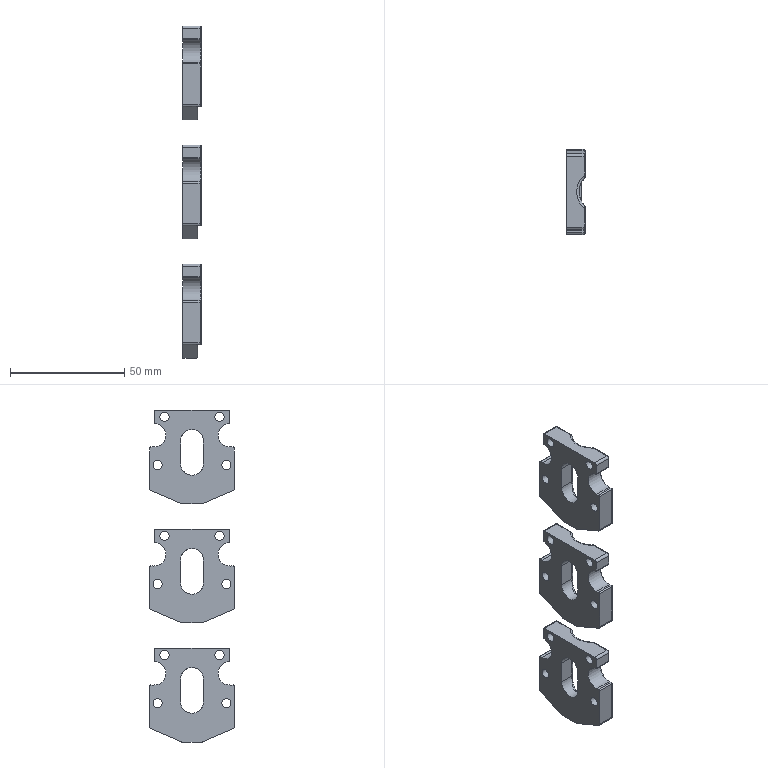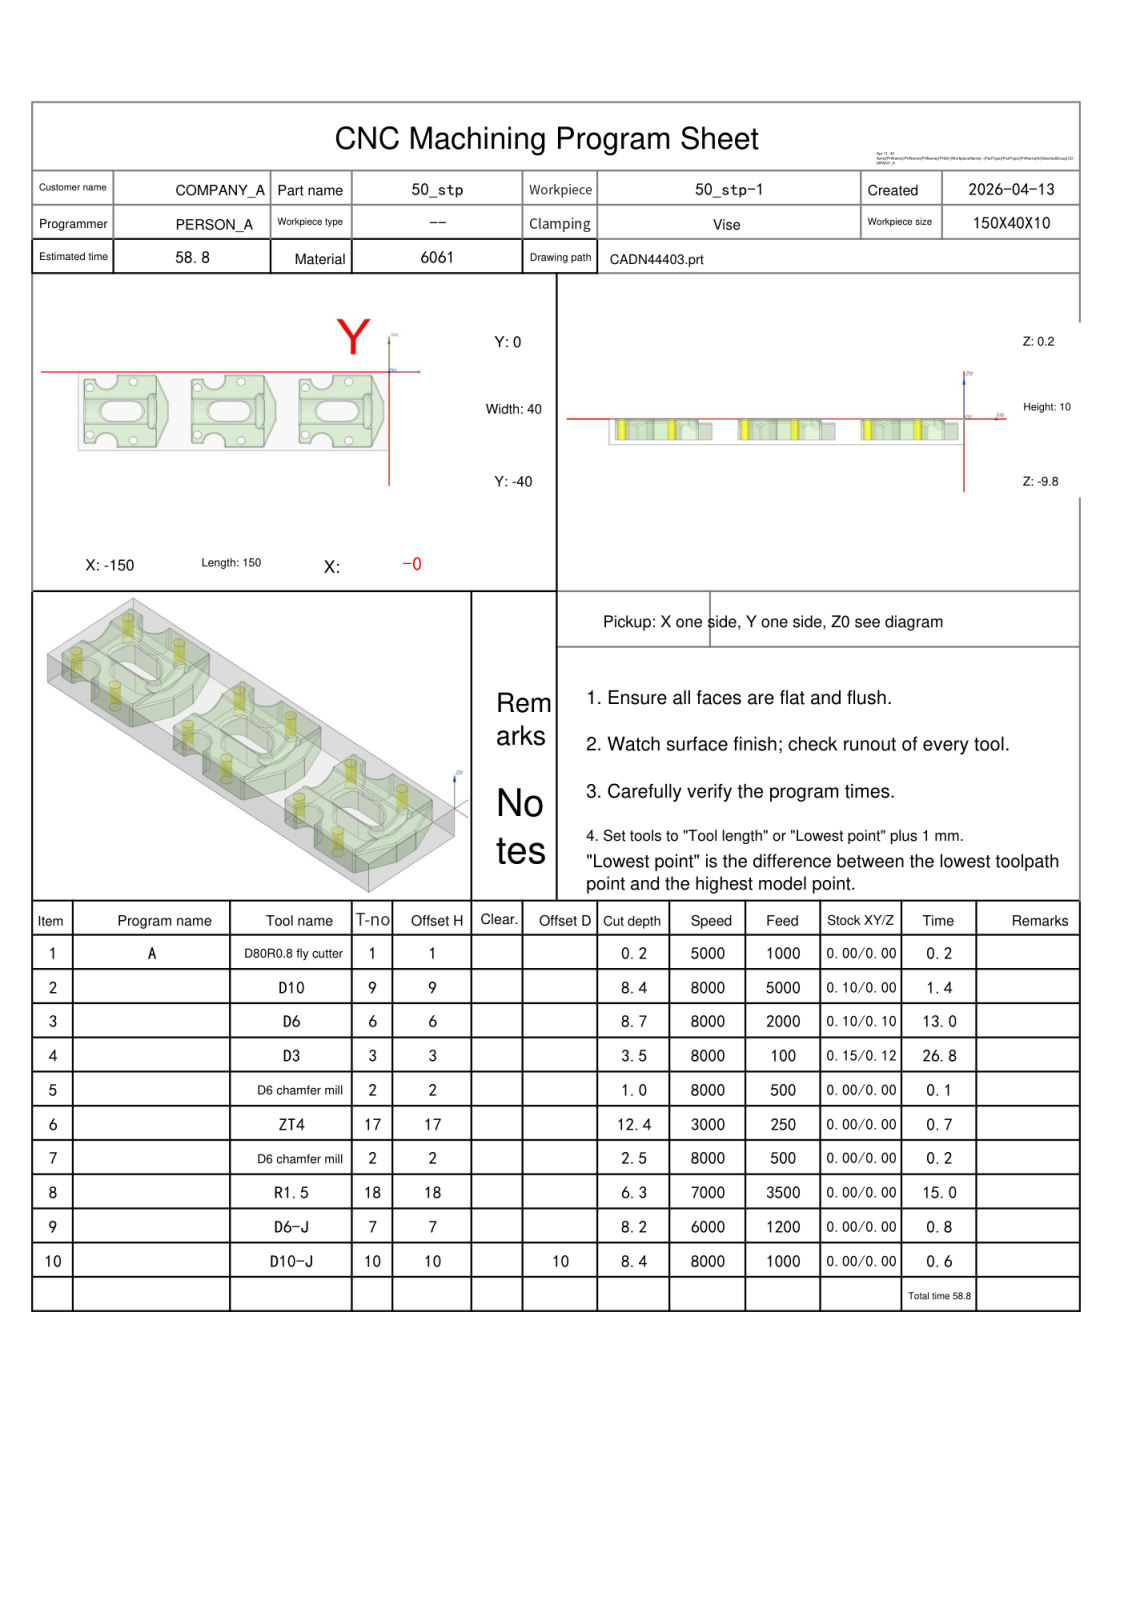NC program | NX | posted by the shop | part box 8 x 37 x 145 mm
Lines 1272 to 2331 of 223411:
N3 T06 M06
(D6  D=6. R=0. H=06 ce=0.10 di=0.10)
G00 G90 G54 X4.879 Y-15.796 M03 S8000
G43 H06 Z10.2
M08
Z.975
G01 Z-.225 F2000.
X4.5
G03 X.3 Y-19.996 I0.0 J-4.2
G01 Y-26.039
X.081 Y-26.55
X-.11 Y-26.995
G02 X-.397 Y-27.298 I-.551 J.236
G01 X-1.104 Y-27.644
G03 X-1.398 Y-27.963 I.264 J-.539
G02 X-2.795 Y-28.916 I-1.396 J.548
X-4.287 Y-27.567 I0.0 J1.5
G01 X-4.66 Y-23.887
X-4.667 Y-23.736
G02 X-3.167 Y-22.236 I1.5 J0.0
X-1.675 Y-23.585 I0.0 J-1.5
G01 X-1.365 Y-26.646
G03 X-1.289 Y-26.883 I.597 J.06
G01 X-.736 Y-27.851
G02 X-.657 Y-28.148 I-.521 J-.298
X-.705 Y-28.385 I-.6 J0.0
G01 X-5.211 Y-38.898
G02 X-5.718 Y-39.859 I-4.039 J1.518
G01 X-5.831 Y-39.78
G03 X-5.688 Y-39.553 I-3.328 J2.279
X-5.198 Y-37.615 I-3.592 J1.938
G01 X-5.2 Y-37.496
Y-29.121
X-5.197 Y-28.968
G03 X-8.5 Y-25.605 I-3.364 J0.0
G01 X-9.376
G03 X-12.749 Y-22.954 I-3.424 J-.885
G01 X-13.466
G02 X-14.063 Y-22.41 I0.0 J.6
G01 X-14.138 Y-21.619
G03 X-14.373 Y-21.197 I-.597 J-.056
G02 X-14.967 Y-20. I.905 J1.196
X-13.469 Y-18.5 I1.5 J0.0
G01 X-9.73 Y-18.497
X-9.729
G02 X-8.229 Y-19.997 I0.0 J-1.5
X-9.728 Y-21.497 I-1.5 J0.0
G01 X-12.219 Y-21.499
G03 X-12.812 Y-22.015 I.001 J-.6
G01 X-12.872 Y-22.438
G02 X-13.466 Y-22.954 I-.594 J.084
G01 X-42.586
G03 X-44.298 Y-23.405 I0.0 J-3.472
X-46.53 Y-27.082 I2.172 J-3.836
G01 X-46.68
Y-27.077
Y-24.633
Y-13.139
Y-12.918
X-46.528
X-46.525 Y-12.967
X-46.37 Y-13.961
X-46.025 Y-14.751
G03 X-42.975 Y-17.019 I3.509 J1.534
G02 X-42.447 Y-17.614 I-.072 J-.596
X-42.518 Y-17.898 I-.6 J0.0
G01 X-42.978 Y-18.756
G03 X-43.042 Y-19.011 I.476 J-.255
X-42.85 Y-19.424 I.54 J0.0
G02 X-42.584 Y-19.997 I-.484 J-.573
X-43.247 Y-20.742 I-.75 J0.0
G03 X-43.553 Y-20.786 I.661 J-5.684
G01 X-43.68 Y-20.797
G02 X-44.43 Y-20.047 I0.0 J.75
G01 Y-19.946
G02 X-44.312 Y-19.543 I.75 J0.0
G01 X-44.247 Y-19.403
X-43.618 Y-17.432
G02 X-43.047 Y-17.014 I.572 J-.182
G01 X-42.975 Y-17.019
G03 X-42.516 Y-17.046 I.459 J3.802
G01 X-12.749
G03 X-9.362 Y-14.395 I-.07 J3.579
G01 X-8.5
G03 X-5.199 Y-11.013 I-.081 J3.381
G01 X-5.2 Y-10.932
Y-2.504
X-5.198 Y-2.367
G03 X-5.689 Y-.445 I-4.005 J0.0
X-5.831 Y-.221 I-3.47 J-2.055
G01 X-5.731 Y-.149
G02 X-5.212 Y-1.101 I-3.568 J-2.562
G01 X-.712 Y-11.599
G02 X-.664 Y-11.835 I-.551 J-.236
X-.743 Y-12.133 I-.6 J0.0
G01 X-1.296 Y-13.102
G03 X-1.372 Y-13.341 I.521 J-.297
G01 X-1.672 Y-16.401
G02 X-3.165 Y-17.755 I-1.493 J.147
X-4.665 Y-16.255 I0.0 J1.5
G01 X-4.658 Y-16.108
X-4.296 Y-12.427
G02 X-2.804 Y-11.073 I1.493 J-.147
X-1.409 Y-12.021 I0.0 J-1.5
G03 X-1.115 Y-12.34 I.558 J.221
G01 X-.404 Y-12.687
G02 X-.116 Y-12.99 I-.264 J-.539
G01 X.228 Y-13.793
X.3 Y-13.961
Y-20.966
G02 X-.226 Y-21.561 I-.6 J0.0
G01 X-3.593 Y-21.981
G03 X-4.009 Y-22.231 I.074 J-.595
G02 X-4.5 Y-22.486 I-.491 J.345
X-4.797 Y-22.407 I0.0 J.6
G03 X-6.613 Y-21.659 I-3.763 J-6.561
G02 X-6.912 Y-21.471 I.156 J.579
G03 X-7.947 Y-20.465 I-5.888 J-5.019
G02 X-8.169 Y-19.998 I.378 J.466
X-7.946 Y-19.532 I.6 J0.0
G03 X-6.906 Y-18.522 I-4.873 J6.065
G02 X-6.608 Y-18.335 I.455 J-.391
G03 X-4.798 Y-17.584 I-1.973 J7.321
G02 X-4.5 Y-17.505 I.298 J-.521
X-3.9 Y-18.104 I0.0 J-.6
G01 Y-21.887
X-3.915 Y-22.021
G02 X-4.207 Y-22.409 I-.585 J.135
G03 X-5.281 Y-24.242 I1.026 J-1.833
X-5.014 Y-25.267 I2.1 J0.0
G01 X4.579 Y-26.509
Z.975
G00 Z3.
G01 X4.879 Y-15.797 F6000.
G00 Z.75
G01 Z-.45 F2000.
X4.5
G03 X.3 Y-19.997 I0.0 J-4.2
G01 Y-26.039
X.081 Y-26.55
X-.382 Y-27.631
G02 X-.701 Y-27.932 I-.506 J.217
G01 X-1.361 Y-28.171
G03 X-1.597 Y-28.327 I.205 J-.564
G02 X-2.698 Y-28.809 I-1.101 J1.018
X-4.184 Y-27.516 I0.0 J1.5
G01 X-4.705 Y-23.77
G02 X-4.72 Y-23.564 I1.486 J.207
X-3.22 Y-22.064 I1.5 J0.0
X-1.734 Y-23.357 I0.0 J-1.5
G01 X-1.213 Y-27.102
G02 X-1.198 Y-27.309 I-1.486 J-.207
G01 X-1.202 Y-27.413
X-1.203 Y-27.451
G03 X-1.157 Y-27.672 I.55 J0.0
G01 X-.879 Y-28.307
G02 X-.828 Y-28.548 I-.549 J-.241
X-.876 Y-28.784 I-.6 J0.0
G01 X-5.211 Y-38.898
G02 X-5.718 Y-39.859 I-4.039 J1.518
G01 X-5.778 Y-39.817
X-5.776 Y-39.811
G03 X-5.2 Y-37.947 I-2.731 J1.864
G01 Y-37.946
Y-37.734
X-5.198 Y-37.615
X-5.2 Y-37.496
Y-29.121
X-5.196 Y-28.964
X-5.2 Y-28.808
Y-28.772
G03 X-8.5 Y-25.436 I-3.336 J0.0
G01 X-9.313
G03 X-12.749 Y-22.707 I-3.483 J-.858
G01 X-42.586
G03 X-45.021 Y-23.656 I0.0 J-3.6
X-46.595 Y-27.082 I3.297 J-3.59
G01 X-46.68 Y-27.079
Y-24.401
Y-13.139
Y-12.918
X-46.595
G03 X-45.73 Y-15.54 I4.991 J.192
X-42.5 Y-17.293 I3.259 J2.154
G01 X-12.749
G03 X-9.315 Y-14.564 I-.039 J3.574
G01 X-8.5
G03 X-6.884 Y-14.121 I-.048 J3.348
X-5.198 Y-11.213 I-1.664 J2.908
G01 X-5.2 Y-11.095
Y-10.932
Y-2.504
X-5.198 Y-2.367
X-5.2 Y-2.23
Y-2.054
Y-2.053
G03 X-5.779 Y-.184 I-3.307 J0.0
G01 X-5.731 Y-.149
G02 X-5.212 Y-1.101 I-3.568 J-2.562
G01 X-.871 Y-11.228
G02 X-.827 Y-11.445 I-.507 J-.217
X-.873 Y-11.667 I-.551 J0.0
G01 X-1.156 Y-12.312
G03 X-1.207 Y-12.553 I.55 J-.241
G01 X-1.206 Y-12.591
X-1.203 Y-12.685
G02 X-1.217 Y-12.89 I-1.5 J0.0
G01 X-1.733 Y-16.636
G02 X-3.219 Y-17.931 I-1.486 J.205
X-4.719 Y-16.431 I0.0 J1.5
X-4.705 Y-16.226 I1.5 J0.0
G01 X-4.189 Y-12.481
G02 X-2.703 Y-11.185 I1.486 J-.205
X-1.596 Y-11.673 I0.0 J-1.5
G03 X-1.377 Y-11.819 I.407 J.372
G01 X-.723 Y-12.056
G02 X-.376 Y-12.383 I-.205 J-.564
G01 X.228 Y-13.793
X.3 Y-13.961
Y-22.997
G02 X-.3 Y-23.597 I-.6 J0.0
X-.568 Y-23.534 I0.0 J.6
G01 X-3.463 Y-22.091
G03 X-3.73 Y-22.028 I-.267 J-.537
X-4.115 Y-22.168 I0.0 J-.6
G02 X-4.5 Y-22.308 I-.385 J.46
X-4.796 Y-22.229 I0.0 J.6
G03 X-6.506 Y-21.515 I-3.74 J-6.543
G02 X-6.804 Y-21.322 I.163 J.577
G03 X-7.65 Y-20.451 I-5.993 J-4.973
G02 X-7.852 Y-20.001 I.398 J.449
X-7.65 Y-19.552 I.6 J0.0
G03 X-6.798 Y-18.674 I-5.139 J5.834
G02 X-6.501 Y-18.481 I.461 J-.384
G03 X-4.797 Y-17.766 I-2.047 J7.266
G02 X-4.5 Y-17.687 I.297 J-.522
X-3.9 Y-18.285 I0.0 J-.6
G01 Y-21.709
X-3.921 Y-21.863
G02 X-4.226 Y-22.241 I-.579 J.156
G03 X-5.365 Y-24.109 I.96 J-1.868
X-5.133 Y-25.069 I2.1 J0.0
G01 X4.579 Y-26.509
Z.75
G00 Z2.775
G01 X4.879 Y-15.794 F6000.
G00 Z.525
G01 Z-.675 F2000.
X4.5
G03 X.3 Y-19.994 I0.0 J-4.2
G01 Y-26.039
X.081 Y-26.55
X-.345 Y-27.543
G02 X-.646 Y-27.829 I-.481 J.206
G01 X-1.265 Y-28.054
G03 X-1.504 Y-28.215 I.205 J-.564
G02 X-2.616 Y-28.708 I-1.112 J1.007
X-4.094 Y-27.458 I0.0 J1.5
G01 X-4.741 Y-23.644
G02 X-4.762 Y-23.393 I1.479 J.251
X-3.262 Y-21.893 I1.5 J0.0
X-1.783 Y-23.142 I0.0 J-1.5
G01 X-1.137 Y-26.957
G02 X-1.116 Y-27.208 I-1.479 J-.251
G01 X-1.121 Y-27.332
X-1.123 Y-27.375
G03 X-1.079 Y-27.585 I.523 J0.0
G01 X-.821 Y-28.175
G02 X-.771 Y-28.415 I-.55 J-.24
X-.819 Y-28.651 I-.6 J0.0
G01 X-5.211 Y-38.898
G02 X-5.718 Y-39.859 I-4.039 J1.518
G01 X-5.777 Y-39.818
X-5.684 Y-39.673
G03 X-5.2 Y-37.953 I-2.816 J1.72
G01 Y-37.946
Y-37.734
X-5.198 Y-37.615
X-5.2 Y-37.496
Y-29.121
X-5.196 Y-28.964
X-5.2 Y-28.808
Y-28.637
Y-28.597
G03 X-8.5 Y-25.258 I-3.34 J0.0
G01 X-9.292
G03 X-12.749 Y-22.44 I-3.556 J-.833
G01 X-42.5
X-42.519
G03 X-44.988 Y-23.362 I0.0 J-3.769
X-46.6 Y-27.068 I3.456 J-3.706
G01 Y-27.082
X-46.601
X-46.68
Y-24.169
Y-13.139
Y-12.918
X-46.6
Y-12.942
G03 X-45.562 Y-16.026 I5.254 J.052
X-42.51 Y-17.56 I3.052 J2.27
G01 X-12.749
G03 X-9.29 Y-14.742 I-.1 J3.655
G01 X-8.5
G03 X-6.89 Y-14.295 I-.071 J3.37
X-5.195 Y-11.367 I-1.68 J2.927
G01 X-5.2 Y-11.192
Y-11.095
Y-10.932
Y-2.504
X-5.198 Y-2.367
X-5.2 Y-2.23
Y-2.047
G03 X-5.641 Y-.403 I-3.3 J-.004
G01 X-5.777 Y-.183
X-5.728 Y-.152
G02 X-5.212 Y-1.101 I-3.571 J-2.559
G01 X-.814 Y-11.363
G02 X-.771 Y-11.57 I-.483 J-.207
X-.815 Y-11.78 I-.526 J0.0
G01 X-1.08 Y-12.387
G03 X-1.13 Y-12.627 I.55 J-.24
G01 X-1.129 Y-12.67
X-1.125 Y-12.78
G02 X-1.145 Y-13.026 I-1.5 J0.0
G01 X-1.781 Y-16.841
G02 X-3.26 Y-18.094 I-1.48 J.246
X-4.76 Y-16.594 I0.0 J1.5
X-4.74 Y-16.348 I1.5 J0.0
G01 X-4.104 Y-12.533
G02 X-2.625 Y-11.28 I1.48 J-.246
X-1.505 Y-11.782 I0.0 J-1.5
G03 X-1.292 Y-11.926 I.392 J.35
G01 X-.683 Y-12.147
G02 X-.337 Y-12.475 I-.205 J-.564
G01 X.228 Y-13.793
X.3 Y-13.961
Y-22.994
G02 X-.3 Y-23.594 I-.6 J0.0
X-.587 Y-23.521 I0.0 J.6
G01 X-3.476 Y-21.95
G03 X-3.763 Y-21.877 I-.286 J-.527
X-4.131 Y-22.004 I0.0 J-.6
G02 X-4.5 Y-22.131 I-.369 J.473
X-4.796 Y-22.052 I0.0 J.6
G03 X-6.442 Y-21.355 I-3.743 J-6.545
G02 X-6.739 Y-21.158 I.169 J.576
G03 X-7.405 Y-20.431 I-6.109 J-4.933
G02 X-7.588 Y-20. I.417 J.431
X-7.405 Y-19.569 I.6 J0.0
G03 X-6.732 Y-18.833 I-5.445 J5.664
G02 X-6.437 Y-18.636 I.466 J-.378
G03 X-4.797 Y-17.936 I-2.134 J7.264
G02 X-4.5 Y-17.857 I.297 J-.521
X-3.9 Y-18.455 I0.0 J-.6
G01 Y-21.532
X-3.926 Y-21.705
G02 X-4.244 Y-22.073 I-.574 J.175
G03 X-5.446 Y-23.972 I.897 J-1.899
X-5.245 Y-24.869 I2.1 J0.0
G01 X4.579 Y-26.509
Z.525
G00 Z2.55
G01 X4.879 Y-15.8 F6000.
G00 Z.3
G01 Z-.9 F2000.
X4.5
G03 X.3 Y-20. I0.0 J-4.2
G01 Y-26.039
X.081 Y-26.55
X-.3 Y-27.439
G02 X-.587 Y-27.71 I-.458 J.196
G01 X-1.166 Y-27.922
G03 X-1.408 Y-28.087 I.206 J-.563
G02 X-2.529 Y-28.59 I-1.121 J.996
X-4. Y-27.382 I0.0 J1.5
G01 X-4.774 Y-23.478
G02 X-4.803 Y-23.186 I1.471 J.292
X-3.303 Y-21.686 I1.5 J0.0
X-1.832 Y-22.894 I0.0 J-1.5
G01 X-1.058 Y-26.799
G02 X-1.029 Y-27.09 I-1.471 J-.292
G01 X-1.036 Y-27.234
X-1.038 Y-27.282
G03 X-.997 Y-27.481 I.498 J0.0
G01 X-.758 Y-28.029
G02 X-.708 Y-28.269 I-.55 J-.239
X-.757 Y-28.505 I-.6 J0.0
G01 X-5.211 Y-38.898
G02 X-5.715 Y-39.854 I-4.039 J1.518
G01 X-5.773 Y-39.813
X-5.684 Y-39.673
G03 X-5.2 Y-37.953 I-2.816 J1.72
G01 Y-37.946
Y-28.459
X-5.199 Y-28.396
G03 X-8.5 Y-25.033 I-3.363 J0.0
G01 X-9.28
G03 X-12.749 Y-22.15 I-3.574 J-.771
G01 X-18.484
X-20. Y-22.182
X-30.
X-31.516 Y-22.15
X-42.5
G03 X-45.6 Y-23.774 I.001 J-3.773
X-45.723 Y-23.951 I4.28 J-3.092
X-46.6 Y-26.854 I4.403 J-2.914
G01 X-46.68
Y-23.911
Y-13.145
X-46.6
Y-13.184
G03 X-45.6 Y-16.226 I5.283 J.05
X-42.5 Y-17.85 I3.101 J2.149
G01 X-31.516
X-30. Y-17.818
X-20.
X-18.484 Y-17.85
X-12.749
G03 X-9.28 Y-14.967 I-.077 J3.622
G01 X-8.5
G03 X-5.199 Y-11.604 I-.063 J3.363
G01 X-5.2 Y-11.541
Y-2.047
G03 X-5.615 Y-.445 I-3.3 J0.0
G01 X-5.774 Y-.188
X-5.725 Y-.157
G02 X-5.212 Y-1.101 I-3.574 J-2.554
G01 X-.74 Y-11.535
G02 X-.699 Y-11.731 I-.458 J-.196
X-.741 Y-11.93 I-.498 J0.0
G01 X-.987 Y-12.496
G03 X-1.036 Y-12.735 I.55 J-.239
G01 X-1.034 Y-12.785
X-1.029 Y-12.91
G02 X-1.058 Y-13.201 I-1.5 J0.0
G01 X-1.832 Y-17.106
G02 X-3.303 Y-18.314 I-1.471 J.292
X-4.803 Y-16.814 I0.0 J1.5
X-4.774 Y-16.522 I1.5 J0.0
G01 X-4. Y-12.618
G02 X-2.529 Y-11.41 I1.471 J-.292
X-1.395 Y-11.927 I0.0 J-1.5
G03 X-1.19 Y-12.069 I.377 J.326
G01 X-.628 Y-12.275
G02 X-.283 Y-12.602 I-.206 J-.563
G01 X.228 Y-13.793
X.3 Y-13.961
Y-23.
G02 X-.3 Y-23.6 I-.6 J0.0
X-.609 Y-23.514 I0.0 J.6
G01 X-3.494 Y-21.778
G03 X-3.804 Y-21.693 I-.309 J-.514
X-4.152 Y-21.804 I0.0 J-.6
G02 X-4.5 Y-21.915 I-.348 J.489
X-4.797 Y-21.837 I0.0 J.6
G03 X-6.38 Y-21.154 I-3.766 J-6.559
G02 X-6.675 Y-20.953 I.175 J.574
G03 X-7.137 Y-20.416 I-6.179 J-4.851
G02 X-7.299 Y-20.006 I.438 J.41
X-7.137 Y-19.596 I.6 J0.0
G03 X-6.662 Y-19.044 I-5.69 J5.368
G02 X-6.367 Y-18.842 I.471 J-.371
G03 X-4.797 Y-18.163 I-2.196 J7.238
G02 X-4.5 Y-18.085 I.297 J-.521
X-3.9 Y-18.682 I0.0 J-.6
G01 Y-21.318
G02 X-3.934 Y-21.514 I-.6 J.002
X-4.266 Y-21.868 I-.566 J.199
G03 X-5.549 Y-23.802 I.818 J-1.934
X-5.383 Y-24.62 I2.1 J0.0
G01 X4.579 Y-26.509
Z.3
G00 Z2.325
G01 X4.879 Y-15.79 F6000.
G00 Z.075
G01 Z-1.125 F2000.
X4.5
G03 X.3 Y-19.99 I0.0 J-4.2
G01 Y-26.039
X.081 Y-26.55
X-.233 Y-27.284
G02 X-.505 Y-27.542 I-.435 J.187
G01 X-1.046 Y-27.74
G03 X-1.291 Y-27.909 I.207 J-.563
G02 X-2.421 Y-28.423 I-1.131 J.986
X-3.884 Y-27.256 I0.0 J1.5
G01 X-4.808 Y-23.199
G02 X-4.845 Y-22.866 I1.463 J.333
X-3.345 Y-21.366 I1.5 J0.0
X-1.883 Y-22.533 I0.0 J-1.5
G01 X-.959 Y-26.59
G02 X-.921 Y-26.923 I-1.463 J-.333
G01 X-.93 Y-27.086
X-.933 Y-27.138
X-.894 Y-27.326
X-.674 Y-27.834
G02 X-.624 Y-28.073 I-.551 J-.239
X-.673 Y-28.309 I-.6 J0.0
G01 X-5.211 Y-38.898
G02 X-5.711 Y-39.849 I-4.039 J1.518
G01 X-5.77 Y-39.808
X-5.684 Y-39.673
G03 X-5.2 Y-37.953 I-2.816 J1.72
G01 Y-37.946
Y-28.459
X-5.199 Y-28.384
X-5.203 Y-28.231
X-5.221 Y-27.891
G03 X-8.5 Y-24.702 I-3.338 J-.153
G01 X-9.296
G03 X-12.749 Y-21.831 I-3.549 J-.757
G01 X-17.484
G02 X-20. Y-22.025 I-7.71 J83.514
G01 X-30.
X-30.481 Y-22.015
X-32.518 Y-21.831
X-42.629
G03 X-45.064 Y-22.849 I0.0 J-3.422
X-46.6 Y-26.592 I3.791 J-3.743
G01 Y-26.609
X-46.68
Y-23.626
Y-16.38
Y-13.312
X-46.6
Y-13.399
G03 X-45.529 Y-16.635 I5.54 J.04
X-42.502 Y-18.169 I3.026 J2.218
G01 X-32.516
X-30.481 Y-17.985
X-30. Y-17.975
X-20.
G02 X-17.482 Y-18.169 I-5.202 J-83.882
G01 X-12.749
G03 X-9.296 Y-15.298 I-.095 J3.628
G01 X-8.5
G03 X-5.198 Y-11.882 I-.116 J3.416
G01 X-5.2 Y-11.769
Y-2.047
G03 X-5.615 Y-.445 I-3.3 J0.0
G01 X-5.771 Y-.193
X-5.721 Y-.162
G02 X-5.212 Y-1.101 I-3.578 J-2.549
G01 X-.654 Y-11.734
X-.616 Y-11.92
X-.655 Y-12.108
X-.884 Y-12.636
G03 X-.933 Y-12.874 I.551 J-.238
G01 X-.931 Y-12.93
X-.924 Y-13.069
G02 X-.962 Y-13.403 I-1.5 J0.0
G01 X-1.885 Y-17.448
G02 X-3.347 Y-18.614 I-1.462 J.334
X-4.847 Y-17.114 I0.0 J1.5
X-4.809 Y-16.78 I1.5 J0.0
G01 X-3.886 Y-12.735
G02 X-2.424 Y-11.569 I1.462 J-.334
X-1.277 Y-12.102 I0.0 J-1.5
G03 X-1.079 Y-12.241 I.362 J.305
G01 X-.56 Y-12.432
G02 X-.215 Y-12.758 I-.207 J-.563
G01 X.228 Y-13.793
X.3 Y-13.961
Y-18.992
G02 X-.157 Y-19.575 I-.6 J0.0
G01 X-3.443 Y-20.38
G03 X-3.9 Y-20.963 I.143 J-.583
G01 Y-20.988
G02 X-4.5 Y-21.585 I-.6 J.002
X-4.797 Y-21.507 I0.0 J.6
G03 X-6.397 Y-20.818 I-3.761 J-6.537
G02 X-6.693 Y-20.617 I.174 J.574
G03 X-6.881 Y-20.387 I-6.152 J-4.842
G02 X-7.022 Y-20. I.459 J.387
X-6.881 Y-19.613 I.6 J0.0
G03 X-6.681 Y-19.368 I-5.964 J5.072
G02 X-6.388 Y-19.167 I.471 J-.372
G03 X-4.799 Y-18.474 I-2.228 J7.285
G02 X-4.5 Y-18.395 I.299 J-.52
X-3.9 Y-18.992 I0.0 J-.6
G01 Y-19.492
G03 X.3 Y-23.692 I4.2 J0.0
G01 X4.879
Z.075
G00 Z2.1
G01 Y-15.792 F6000.
G00 Z-.15
G01 Z-1.35 F2000.
X4.5
G03 X.3 Y-19.992 I0.0 J-4.2
G01 Y-26.039
X.081 Y-26.55
X0.0 Y-26.739
G02 X-.337 Y-27.057 I-.535 J.23
G01 X-1.049 Y-27.313
G03 X-1.281 Y-27.465 I.203 J-.564
G02 X-2.37 Y-27.933 I-1.089 J1.032
X-3.83 Y-26.777 I0.0 J1.5
G01 X-4.829 Y-22.539
G02 X-4.869 Y-22.194 I1.46 J.344
X-3.369 Y-20.694 I1.5 J0.0
X-1.909 Y-21.85 I0.0 J-1.5
G01 X-.91 Y-26.089
G02 X-.87 Y-26.433 I-1.46 J-.344
G01 X-.872 Y-26.513
X-.873 Y-26.543
G03 X-.823 Y-26.778 I.582 J0.0
G01 X-.519 Y-27.467
G02 X-.468 Y-27.709 I-.549 J-.242
X-.517 Y-27.945 I-.6 J0.0
G01 X-5.211 Y-38.898
G02 X-5.707 Y-39.843 I-4.039 J1.518
G01 X-5.767 Y-39.802
X-5.684 Y-39.673
G03 X-5.246 Y-38.5 I-2.816 J1.72
X-5.2 Y-37.953 I-3.254 J.547
G01 Y-37.946
Y-28.459
Y-28.333
Y-27.93
X-5.261 Y-27.204
G03 X-8.646 Y-23.979 I-3.384 J-.163
X-9.386 Y-24.061 I0.0 J-3.388
X-12.749 Y-21.496 I-3.457 J-1.045
G01 X-16.79
X-18.362 Y-21.715
X-19.44 Y-21.913
G02 X-19.737 Y-21.94 I-.298 J1.62
G01 X-30.012
G02 X-31.266 Y-21.786 I0.0 J5.172
G01 X-31.548 Y-21.715
X-33.211 Y-21.496
X-42.506
G03 X-45.302 Y-22.797 I0.0 J-3.657
X-46.6 Y-26.351 I4.219 J-3.554
G01 Y-26.357
X-46.68
Y-23.337
Y-13.643
X-46.601
X-46.6 Y-13.649
G03 X-45.302 Y-17.203 I5.517 J0.0
X-42.506 Y-18.504 I2.797 J2.356
G01 X-33.21
X-31.549 Y-18.285
X-31.266 Y-18.214
G02 X-30.01 Y-18.06 I1.256 J-5.029
G01 X-20.
G02 X-18.737 Y-18.216 I-.125 J-6.194
G01 X-18.39 Y-18.285
X-16.789 Y-18.504
X-12.749
G03 X-9.367 Y-15.894 I-.101 J3.628
G01 X-9.295 Y-15.892
X-8.866 Y-16.
X-8.5
G03 X-5.261 Y-12.796 I-.142 J3.383
G01 X-5.2 Y-12.07
Y-11.995
X-5.198 Y-11.882
X-5.2 Y-11.769
Y-2.047
G03 X-5.615 Y-.445 I-3.3 J0.0
G01 X-5.768 Y-.198
X-5.717 Y-.167
G02 X-5.212 Y-1.101 I-3.581 J-2.544
G01 X-.517 Y-12.056
G02 X-.47 Y-12.283 I-.531 J-.228
X-.519 Y-12.517 I-.578 J0.0
G01 X-.821 Y-13.202
G03 X-.872 Y-13.444 I.549 J-.242
G01 X-.871 Y-13.476
X-.869 Y-13.555
G02 X-.909 Y-13.899 I-1.5 J0.0
G01 X-1.909 Y-18.134
G02 X-3.369 Y-19.289 I-1.46 J.345
X-4.869 Y-17.789 I0.0 J1.5
X-4.829 Y-17.445 I1.5 J0.0
G01 X-3.829 Y-13.21
G02 X-2.369 Y-12.055 I1.46 J-.345
X-1.277 Y-12.527 I0.0 J-1.5
G03 X-1.051 Y-12.675 I.421 J.396
G01 X-.35 Y-12.927
G02 X-.002 Y-13.255 I-.204 J-.564
G01 X.228 Y-13.793
X.3 Y-13.961
Y-19.675
G02 X-.294 Y-20.275 I-.6 J0.0
G01 X-3.466 Y-20.305
G03 X-3.98 Y-20.605 I.006 J-.6
G02 X-4.5 Y-20.906 I-.52 J.299
X-4.802 Y-20.825 I0.0 J.6
G03 X-5.352 Y-20.531 I-3.844 J-6.542
G02 X-5.689 Y-19.992 I.263 J.539
X-5.352 Y-19.452 I.6 J0.0
G03 X-4.802 Y-19.159 I-3.291 J6.835
G02 X-4.5 Y-19.078 I.302 J-.519
X-3.9 Y-19.675 I0.0 J-.6
G01 Y-20.175
G03 X.3 Y-24.375 I4.2 J0.0
G01 X4.879
Z-.15
G00 Z1.875
G01 Y-19.992 F6000.
G00 Z-.397
G01 Z-1.597 F2000.
X.485
Y-15.603
G03 X.203 Y-14.23 I-3.485 J0.0
G01 X-5.241 Y-1.526
G03 X-5.656 Y-.379 I-3.257 J-.528
G01 X-5.764 Y-.204
X-5.713 Y-.173
G02 X-5.212 Y-1.101 I-3.585 J-2.538
G01 X.228 Y-13.793
X.3 Y-13.961
X.385 Y-14.161
X.6 Y-14.845
X.679 Y-15.54
Y-24.469
X.597 Y-25.17
X.375 Y-25.864
X.3 Y-26.039
X.081 Y-26.55
X-5.211 Y-38.898
G02 X-5.704 Y-39.838 I-4.039 J1.518
G01 X-5.763 Y-39.797
X-5.684 Y-39.673
G03 X-5.241 Y-38.474 I-2.816 J1.72
G01 X.203 Y-25.77
G03 X.485 Y-24.397 I-3.203 J1.373
G01 Y-19.992
Y-19.492
Z-.397
G00 Z1.65
G01 X4.879 Y-19.992 F6000.
G00 Z-.643
G01 Z-1.843 F2000.
X.59
Y-15.603
G03 X.3 Y-14.188 I-3.59 J0.0
G01 X-5.4 Y-.889
G03 X-5.499 Y-.674 I-3.76 J-1.611
X-5.615 Y-.445 I-3.001 J-1.373
G01 X-5.76 Y-.21
X-5.712 Y-.175
G02 X-5.212 Y-1.101 I-3.587 J-2.536
G01 X.228 Y-13.793
X.3 Y-13.961
X.385 Y-14.161
X.6 Y-14.845
X.679 Y-15.54
Y-24.469
X.597 Y-25.17
X.375 Y-25.864
X.3 Y-26.039
X.081 Y-26.55
X-5.211 Y-38.898
G02 X-5.7 Y-39.832 I-4.039 J1.518
G01 X-5.759 Y-39.791
X-5.684 Y-39.673
G03 X-5.499 Y-39.326 I-2.816 J1.72
X-5.4 Y-39.111 I-3.66 J1.826
G01 X.3 Y-25.812
G03 X.59 Y-24.397 I-3.3 J1.414
G01 Y-19.992
Y-19.492
Z-.643
G00 Z1.65
G01 X-44.4 Y-21.197 F6000.
G00 Z.15
G02 X-44.4 Y-21.197 Z-.133 I-2.28 J1.207 F2000.
X-44.4 Y-21.197 Z-.416 I-2.28 J1.207
X-44.4 Y-21.197 Z-.699 I-2.28 J1.207
X-44.4 Y-21.197 Z-.982 I-2.28 J1.207
X-44.4 Y-21.197 Z-1.265 I-2.28 J1.207
X-44.4 Y-21.197 Z-1.548 I-2.28 J1.207
X-46.68 Y-22.57 Z-1.597 I-2.28 J1.207
G01 Y-19.99
Y-13.896
X-46.601
G03 X-45.81 Y-16.912 I6.228 J.02
X-42.5 Y-18.956 I3.373 J1.76
G01 X-33.901
G03 X-31.383 Y-18.391 I-.52 J8.215
G02 X-30. Y-18.099 I1.565 J-3.991
G01 X-20.
G02 X-18.737 Y-18.355 I-.119 J-3.834
G03 X-16.099 Y-18.956 I3.328 J8.514
G01 X-12.749
X-11.395 Y-18.672
Y-21.328
X-12.749 Y-21.044
X-16.099
G03 X-18.737 Y-21.645 I.723 J-9.262
G02 X-19.999 Y-21.901 I-1.262 J2.984
G01 X-20.
X-30.
G02 X-31.382 Y-21.609 I.155 J4.153
G03 X-33.901 Y-21.044 I-3.039 J-7.65
G01 X-42.632
G03 X-45.086 Y-22.127 I0.0 J-3.322
X-46.603 Y-26.041 I4.291 J-3.915
G01 Y-26.084
X-46.68
Y-19.99
Y-19.49
G03 X-50.88 Y-15.29 I-4.2 J0.0
G01 Z-.397
G00 Z1.65
G01 X-44.712 Y-21.017 F6000.
G00 Z-.097
G02 X-44.712 Y-21.017 Z-.34 I-1.968 J1.027 F2000.
X-44.712 Y-21.017 Z-.584 I-1.968 J1.027
X-44.712 Y-21.017 Z-.827 I-1.968 J1.027
X-44.712 Y-21.017 Z-1.07 I-1.968 J1.027
X-44.712 Y-21.017 Z-1.314 I-1.968 J1.027
X-44.712 Y-21.017 Z-1.557 I-1.968 J1.027
X-44.712 Y-21.017 Z-1.801 I-1.968 J1.027
X-46.68 Y-22.21 Z-1.843 I-1.968 J1.027
G01 Y-19.99
Y-14.179
X-46.6
Y-14.229
G03 X-45.679 Y-17.584 I6.572 J0.0
X-42.5 Y-19.461 I3.217 J1.818
G01 X-34.481
G03 X-32.554 Y-19.025 I-.097 J4.909
G02 X-30.57 Y-18.187 I9.363 J-19.4
X-30.272 Y-18.12 I.57 J-1.813
G01 X-30. Y-18.1
X-20.
G02 X-18.17 Y-18.693 I-.705 J-5.298
G03 X-15.519 Y-19.461 I2.977 J5.314
G01 X-12.749
X-12.519 Y-19.462
X-11.527 Y-19.22
X-11.4 Y-19.169
Y-20.831
X-11.527 Y-20.78
X-12.519 Y-20.538
X-12.749 Y-20.539
X-15.519
G03 X-18.19 Y-21.314 I.339 J-6.157
G02 X-20. Y-21.9 I-2.418 J4.378
G01 X-30.02
X-30.24 Y-21.885
G02 X-30.57 Y-21.813 I.24 J1.885
X-32.014 Y-21.209 I3.297 J9.909
G03 X-34.481 Y-20.539 I-2.836 J-5.567
G01 X-42.5
G03 X-45.679 Y-22.416 I.038 J-3.695
X-46.6 Y-25.73 I5.647 J-3.354
G01 X-46.68
Y-19.99
Y-19.49
G03 X-50.88 Y-15.29 I-4.2 J0.0
G01 Z-.643
G00 Z3.
G01 X-22.396 Y-20.9 F6000.
G00 Z-.343
G01 X-20.064 Z-.384 F2000.
X-19.834 Y-20.868 Z-.388
X-19.598 Y-20.805 Z-.392
X-19.374 Y-20.708 Z-.396
X-18.181 Y-19.992 Z-.421
X-19.415 Y-19.277 Z-.446
X-19.589 Y-19.199 Z-.449
X-19.827 Y-19.136 Z-.453
X-20.07 Y-19.1 Z-.457
X-28.748 Z-.609
X-20.07 Z-.76
X-19.827 Y-19.136 Z-.765
X-19.559 Y-19.213 Z-.77
X-19.415 Y-19.277 Z-.772
X-18.181 Y-19.992 Z-.797
X-19.374 Y-20.708 Z-.822
X-19.608 Y-20.81 Z-.826
X-19.834 Y-20.868 Z-.83
X-20.064 Y-20.9 Z-.834
X-24.13 Z-.905
X-20.064 Z-.976
X-19.834 Y-20.868 Z-.98
X-19.598 Y-20.805 Z-.984
X-19.374 Y-20.708 Z-.989
X-18.181 Y-19.992 Z-1.013
X-19.415 Y-19.277 Z-1.038
X-19.589 Y-19.199 Z-1.041
X-19.827 Y-19.136 Z-1.045
X-20.07 Y-19.1 Z-1.05
X-28.748 Z-1.201
X-20.07 Z-1.353
X-19.827 Y-19.136 Z-1.357
X-19.559 Y-19.213 Z-1.362
X-19.415 Y-19.277 Z-1.365
X-18.181 Y-19.992 Z-1.39
X-19.374 Y-20.708 Z-1.414
X-19.608 Y-20.81 Z-1.418
X-19.834 Y-20.868 Z-1.422
X-20.064 Y-20.9 Z-1.426
X-24.13 Z-1.497
X-20.064 Z-1.568
X-19.834 Y-20.868 Z-1.572
X-19.598 Y-20.805 Z-1.577
X-19.374 Y-20.708 Z-1.581
X-18.181 Y-19.992 Z-1.605
X-19.415 Y-19.277 Z-1.63
X-19.589 Y-19.199 Z-1.633
X-19.827 Y-19.136 Z-1.638
X-20.07 Y-19.1 Z-1.642
X-28.748 Z-1.794
X-20.07 Z-1.945
X-19.827 Y-19.136 Z-1.949
X-19.559 Y-19.213 Z-1.954
X-19.415 Y-19.277 Z-1.957
X-18.181 Y-19.992 Z-1.982
X-19.374 Y-20.708 Z-2.006
X-19.608 Y-20.81 Z-2.011
X-19.834 Y-20.868 Z-2.015
X-20.064 Y-20.9 Z-2.019
X-24.13 Z-2.09
Y-21.9
X-30.02
X-30.24 Y-21.885
G02 X-30.849 Y-21.7 I.24 J1.885
G01 X-31.039 Y-21.615
X-32.715 Y-20.622
G03 X-34.331 Y-20. I-2.645 J-4.464
X-32.554 Y-19.295 I-1.181 J5.575
G01 X-31.077 Y-18.399
X-30.849 Y-18.3
X-30.746 Y-18.253
X-30.57 Y-18.187
G02 X-30.272 Y-18.12 I.57 J-1.813
G01 X-30. Y-18.1
X-20.
G02 X-19.244 Y-18.257 I-.705 J-5.298
G01 X-19.151 Y-18.3
X-18.96 Y-18.385
X-17.08 Y-19.474
G03 X-15.662 Y-20. I2.243 J3.873
G01 X-15.974 Y-20.062
X-17.355 Y-20.664
X-18.919 Y-21.6
X-19.151 Y-21.7
X-19.275 Y-21.756
G02 X-20. Y-21.9 I-1.332 J4.821
G01 X-24.13
X-24.63
Z-.89
G00 Z1.157
G01 X-22.394 Y-20.9 F6000.
G00 Z-.59
G01 X-20.064 Z-.63 F2000.
X-19.834 Y-20.868 Z-.634
X-19.608 Y-20.81 Z-.638
X-19.55 Y-20.782 Z-.64
X-19.313 Y-20.626 Z-.645
X-18.489 Y-20.004 Z-.663
X-19.322 Y-19.368 Z-.681
X-19.59 Y-19.199 Z-.686
X-19.827 Y-19.136 Z-.691
X-20.07 Y-19.1 Z-.695
X-29.268 Z-.856
X-20.07 Z-1.016
X-19.827 Y-19.136 Z-1.02
X-19.59 Y-19.199 Z-1.025
X-19.322 Y-19.368 Z-1.03
X-18.489 Y-20.004 Z-1.048
X-19.313 Y-20.626 Z-1.066
X-19.55 Y-20.782 Z-1.071
X-19.608 Y-20.81 Z-1.073
X-19.834 Y-20.868 Z-1.077
X-20.064 Y-20.9 Z-1.081
X-24.13 Z-1.152
X-20.064 Z-1.223
X-19.834 Y-20.868 Z-1.227
X-19.608 Y-20.81 Z-1.231
X-19.55 Y-20.782 Z-1.232
X-19.313 Y-20.626 Z-1.237
X-18.489 Y-20.004 Z-1.255
X-19.322 Y-19.368 Z-1.273
X-19.59 Y-19.199 Z-1.279
X-19.827 Y-19.136 Z-1.283
X-20.07 Y-19.1 Z-1.287
X-29.268 Z-1.448
X-20.07 Z-1.608
X-19.827 Y-19.136 Z-1.613
X-19.59 Y-19.199 Z-1.617
X-19.322 Y-19.368 Z-1.622
X-18.489 Y-20.004 Z-1.641
X-19.313 Y-20.626 Z-1.659
X-19.55 Y-20.782 Z-1.664
X-19.608 Y-20.81 Z-1.665
X-19.834 Y-20.868 Z-1.669
X-20.064 Y-20.9 Z-1.673
X-24.13 Z-1.744
X-20.064 Z-1.815
X-19.834 Y-20.868 Z-1.819
X-19.608 Y-20.81 Z-1.823
X-19.55 Y-20.782 Z-1.824
X-19.313 Y-20.626 Z-1.829
X-18.489 Y-20.004 Z-1.847
X-19.322 Y-19.368 Z-1.865
X-19.59 Y-19.199 Z-1.871
X-19.827 Y-19.136 Z-1.875
X-20.07 Y-19.1 Z-1.88
X-29.268 Z-2.04
X-20.07 Z-2.201
X-19.827 Y-19.136 Z-2.205
X-19.59 Y-19.199 Z-2.209
X-19.322 Y-19.368 Z-2.215
X-18.489 Y-20.004 Z-2.233
X-19.313 Y-20.626 Z-2.251
X-19.55 Y-20.782 Z-2.256
X-19.608 Y-20.81 Z-2.257
X-19.834 Y-20.868 Z-2.261
X-20.064 Y-20.9 Z-2.265
X-24.13 Z-2.336
Y-21.9
X-30.02
X-30.24 Y-21.885
G02 X-31.029 Y-21.597 I.24 J1.885
G01 X-31.413 Y-21.352
X-33.146 Y-19.992
X-32.208 Y-19.303
G02 X-30.981 Y-18.373 I4.993 J-5.315
X-30.746 Y-18.253 I.981 J-1.627
G01 X-30.57 Y-18.187
G02 X-30.272 Y-18.12 I.57 J-1.813
G01 X-30. Y-18.1
X-20.
G02 X-19.244 Y-18.257 I-.705 J-5.298
X-18.972 Y-18.402 I-.756 J-1.743
G01 X-18.744 Y-18.551
X-16.835 Y-20.008
X-18.737 Y-21.444
X-18.937 Y-21.575
G02 X-19.275 Y-21.756 I-1.063 J1.575
X-20. Y-21.9 I-1.332 J4.821
G01 X-24.13
X-24.63
Z-1.136
G00 Z.91
G01 X-22.364 Y-20.9 F6000.
G00 Z-.836
G01 X-20.064 Z-.876 F2000.
X-19.834 Y-20.868 Z-.88
X-19.608 Y-20.81 Z-.884
X-19.52 Y-20.767 Z-.886
X-19.032 Y-20.382 Z-.897
X-18.673 Y-20.001 Z-.906
X-19.064 Y-19.587 Z-.916
X-19.552 Y-19.218 Z-.927
X-19.59 Y-19.199 Z-.928
X-19.827 Y-19.136 Z-.932
X-20.07 Y-19.1 Z-.936
X-29.552 Z-1.102
X-20.07 Z-1.267